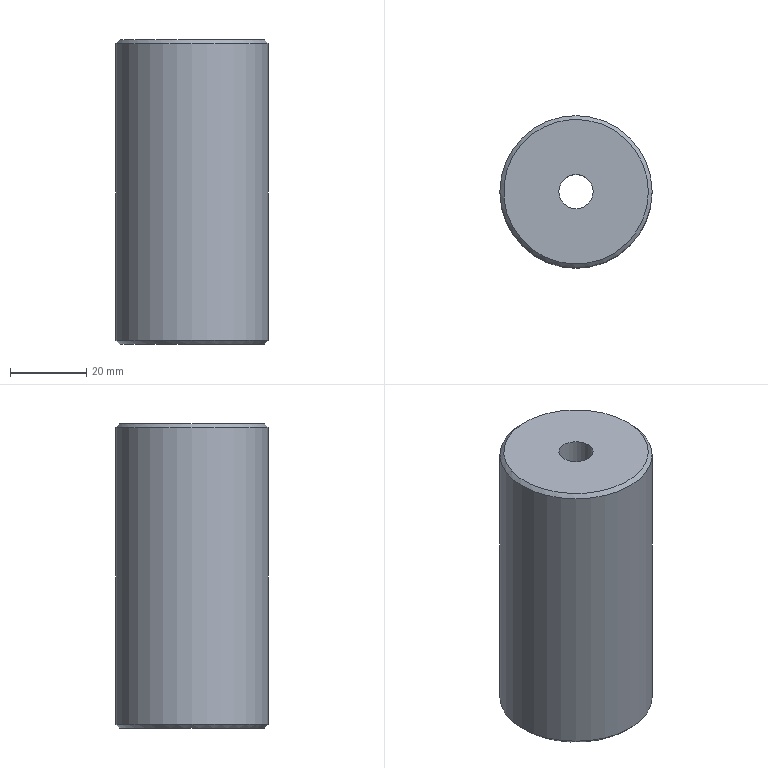Part | STEP file | gslz 2016.10.28-6_id174_x_t | 1 solid | 8 faces | box 40 x 40 x 80 mm | volume 91705 mm3 | cylinder 3 | plane 3 | cone 2 | commonest cylinder face diameters 9 x1 14 x1 40 x1
STEP:
#1=CARTESIAN_POINT('',(-220.,150.,50.992));
#2=VERTEX_POINT('',#1);
#3=CARTESIAN_POINT('',(-240.,150.,50.992));
#4=DIRECTION('',(0.,0.,-1.));
#5=DIRECTION('',(1.,0.,0.));
#6=AXIS2_PLACEMENT_3D('',#3,#4,#5);
#7=CIRCLE('',#6,20.);
#8=EDGE_CURVE('',#2,#2,#7,.T.);
#9=ORIENTED_EDGE('',*,*,#8,.F.);
#10=EDGE_LOOP('',(#9));
#11=FACE_BOUND('',#10,.T.);
#12=CARTESIAN_POINT('',(-220.,150.,128.992));
#13=VERTEX_POINT('',#12);
#14=CARTESIAN_POINT('',(-240.,150.,128.992));
#15=DIRECTION('',(0.,0.,1.));
#16=DIRECTION('',(1.,0.,0.));
#17=AXIS2_PLACEMENT_3D('',#14,#15,#16);
#18=CIRCLE('',#17,20.);
#19=EDGE_CURVE('',#13,#13,#18,.T.);
#20=ORIENTED_EDGE('',*,*,#19,.F.);
#21=EDGE_LOOP('',(#20));
#22=FACE_BOUND('',#21,.T.);
#23=CARTESIAN_POINT('',(-240.,150.,147.99));
#24=DIRECTION('',(0.,0.,-1.));
#25=DIRECTION('',(-1.,0.,0.));
#26=AXIS2_PLACEMENT_3D('',#23,#24,#25);
#27=CYLINDRICAL_SURFACE('',#26,20.);
#28=ADVANCED_FACE('',(#11,#22),#27,.T.);
#29=CARTESIAN_POINT('',(-235.5,150.,129.992));
#30=VERTEX_POINT('',#29);
#31=CARTESIAN_POINT('',(-240.,150.,129.992));
#32=DIRECTION('',(0.,0.,1.));
#33=DIRECTION('',(1.,0.,0.));
#34=AXIS2_PLACEMENT_3D('',#31,#32,#33);
#35=CIRCLE('',#34,4.5);
#36=EDGE_CURVE('',#30,#30,#35,.T.);
#37=ORIENTED_EDGE('',*,*,#36,.F.);
#38=EDGE_LOOP('',(#37));
#39=FACE_BOUND('',#38,.T.);
#40=CARTESIAN_POINT('',(-221.,150.,129.992));
#41=VERTEX_POINT('',#40);
#42=CARTESIAN_POINT('',(-240.,150.,129.992));
#43=DIRECTION('',(0.,0.,-1.));
#44=DIRECTION('',(1.,0.,0.));
#45=AXIS2_PLACEMENT_3D('',#42,#43,#44);
#46=CIRCLE('',#45,19.);
#47=EDGE_CURVE('',#41,#41,#46,.T.);
#48=ORIENTED_EDGE('',*,*,#47,.F.);
#49=EDGE_LOOP('',(#48));
#50=FACE_BOUND('',#49,.T.);
#51=CARTESIAN_POINT('',(-505.404,329.404,129.992));
#52=DIRECTION('',(0.,0.,-1.));
#53=DIRECTION('',(-1.,0.,0.));
#54=AXIS2_PLACEMENT_3D('',#51,#52,#53);
#55=PLANE('',#54);
#56=ADVANCED_FACE('',(#39,#50),#55,.F.);
#57=CARTESIAN_POINT('',(-233.,150.,49.992));
#58=VERTEX_POINT('',#57);
#59=CARTESIAN_POINT('',(-240.,150.,49.992));
#60=DIRECTION('',(0.,0.,1.));
#61=DIRECTION('',(1.,0.,0.));
#62=AXIS2_PLACEMENT_3D('',#59,#60,#61);
#63=CIRCLE('',#62,7.);
#64=EDGE_CURVE('',#58,#58,#63,.T.);
#65=ORIENTED_EDGE('',*,*,#64,.T.);
#66=EDGE_LOOP('',(#65));
#67=FACE_BOUND('',#66,.T.);
#68=CARTESIAN_POINT('',(-221.,150.,49.992));
#69=VERTEX_POINT('',#68);
#70=CARTESIAN_POINT('',(-240.,150.,49.992));
#71=DIRECTION('',(0.,0.,1.));
#72=DIRECTION('',(1.,0.,0.));
#73=AXIS2_PLACEMENT_3D('',#70,#71,#72);
#74=CIRCLE('',#73,19.);
#75=EDGE_CURVE('',#69,#69,#74,.T.);
#76=ORIENTED_EDGE('',*,*,#75,.F.);
#77=EDGE_LOOP('',(#76));
#78=FACE_BOUND('',#77,.T.);
#79=CARTESIAN_POINT('',(-505.404,329.404,49.992));
#80=DIRECTION('',(0.,0.,-1.));
#81=DIRECTION('',(-1.,0.,0.));
#82=AXIS2_PLACEMENT_3D('',#79,#80,#81);
#83=PLANE('',#82);
#84=ADVANCED_FACE('',(#67,#78),#83,.T.);
#85=ORIENTED_EDGE('',*,*,#75,.T.);
#86=EDGE_LOOP('',(#85));
#87=FACE_BOUND('',#86,.T.);
#88=ORIENTED_EDGE('',*,*,#8,.T.);
#89=EDGE_LOOP('',(#88));
#90=FACE_BOUND('',#89,.T.);
#91=CARTESIAN_POINT('',(-240.,150.,50.992));
#92=DIRECTION('',(0.,0.,1.));
#93=DIRECTION('',(-1.,0.,0.));
#94=AXIS2_PLACEMENT_3D('',#91,#92,#93);
#95=CONICAL_SURFACE('',#94,20.,45.);
#96=ADVANCED_FACE('',(#87,#90),#95,.T.);
#97=ORIENTED_EDGE('',*,*,#19,.T.);
#98=EDGE_LOOP('',(#97));
#99=FACE_BOUND('',#98,.T.);
#100=ORIENTED_EDGE('',*,*,#47,.T.);
#101=EDGE_LOOP('',(#100));
#102=FACE_BOUND('',#101,.T.);
#103=CARTESIAN_POINT('',(-240.,150.,129.992));
#104=DIRECTION('',(0.,0.,-1.));
#105=DIRECTION('',(-1.,0.,0.));
#106=AXIS2_PLACEMENT_3D('',#103,#104,#105);
#107=CONICAL_SURFACE('',#106,19.,45.);
#108=ADVANCED_FACE('',(#99,#102),#107,.T.);
#109=ORIENTED_EDGE('',*,*,#36,.T.);
#110=EDGE_LOOP('',(#109));
#111=FACE_BOUND('',#110,.T.);
#112=CARTESIAN_POINT('',(-235.5,150.,89.992));
#113=VERTEX_POINT('',#112);
#114=CARTESIAN_POINT('',(-240.,150.,89.992));
#115=DIRECTION('',(0.,0.,-1.));
#116=DIRECTION('',(1.,0.,0.));
#117=AXIS2_PLACEMENT_3D('',#114,#115,#116);
#118=CIRCLE('',#117,4.5);
#119=EDGE_CURVE('',#113,#113,#118,.T.);
#120=ORIENTED_EDGE('',*,*,#119,.T.);
#121=EDGE_LOOP('',(#120));
#122=FACE_BOUND('',#121,.T.);
#123=CARTESIAN_POINT('',(-240.,150.,129.992));
#124=DIRECTION('',(0.,0.,1.));
#125=DIRECTION('',(1.,0.,0.));
#126=AXIS2_PLACEMENT_3D('',#123,#124,#125);
#127=CYLINDRICAL_SURFACE('',#126,4.5);
#128=ADVANCED_FACE('',(#111,#122),#127,.F.);
#129=ORIENTED_EDGE('',*,*,#119,.F.);
#130=EDGE_LOOP('',(#129));
#131=FACE_BOUND('',#130,.T.);
#132=CARTESIAN_POINT('',(-233.,150.,89.992));
#133=VERTEX_POINT('',#132);
#134=CARTESIAN_POINT('',(-240.,150.,89.992));
#135=DIRECTION('',(0.,0.,-1.));
#136=DIRECTION('',(1.,0.,0.));
#137=AXIS2_PLACEMENT_3D('',#134,#135,#136);
#138=CIRCLE('',#137,7.);
#139=EDGE_CURVE('',#133,#133,#138,.T.);
#140=ORIENTED_EDGE('',*,*,#139,.T.);
#141=EDGE_LOOP('',(#140));
#142=FACE_BOUND('',#141,.T.);
#143=CARTESIAN_POINT('',(-240.,150.,89.992));
#144=DIRECTION('',(0.,0.,1.));
#145=DIRECTION('',(-1.,0.,0.));
#146=AXIS2_PLACEMENT_3D('',#143,#144,#145);
#147=PLANE('',#146);
#148=ADVANCED_FACE('',(#131,#142),#147,.F.);
#149=ORIENTED_EDGE('',*,*,#139,.F.);
#150=EDGE_LOOP('',(#149));
#151=FACE_BOUND('',#150,.T.);
#152=ORIENTED_EDGE('',*,*,#64,.F.);
#153=EDGE_LOOP('',(#152));
#154=FACE_BOUND('',#153,.T.);
#155=CARTESIAN_POINT('',(-240.,150.,59.992));
#156=DIRECTION('',(0.,0.,1.));
#157=DIRECTION('',(1.,0.,0.));
#158=AXIS2_PLACEMENT_3D('',#155,#156,#157);
#159=CYLINDRICAL_SURFACE('',#158,7.);
#160=ADVANCED_FACE('',(#151,#154),#159,.F.);
#161=CLOSED_SHELL('',(#28,#56,#84,#96,#108,#128,#148,#160));
#162=MANIFOLD_SOLID_BREP('',#161);
#163=(LENGTH_UNIT()NAMED_UNIT(*)SI_UNIT(.MILLI.,.METRE.));
#164=UNCERTAINTY_MEASURE_WITH_UNIT(LENGTH_MEASURE(0.00002),#163,'','');
#165=(NAMED_UNIT(*)PLANE_ANGLE_UNIT()SI_UNIT($,.RADIAN.));
#166=PLANE_ANGLE_MEASURE_WITH_UNIT(PLANE_ANGLE_MEASURE(0.01745),#165);
#167=DIMENSIONAL_EXPONENTS(0.,0.,0.,0.,0.,0.,0.);
#168=(CONVERSION_BASED_UNIT('DEGREE',#166)NAMED_UNIT(#167)PLANE_ANGLE_UNIT());
#169=(NAMED_UNIT(*)SI_UNIT($,.STERADIAN.)SOLID_ANGLE_UNIT());
#170=(GEOMETRIC_REPRESENTATION_CONTEXT(3)GLOBAL_UNCERTAINTY_ASSIGNED_CONTEXT((#164))GLOBAL_UNIT_ASSIGNED_CONTEXT((#163,#168,#169))REPRESENTATION_CONTEXT('',''));
#171=ADVANCED_BREP_SHAPE_REPRESENTATION('',(#162),#170);